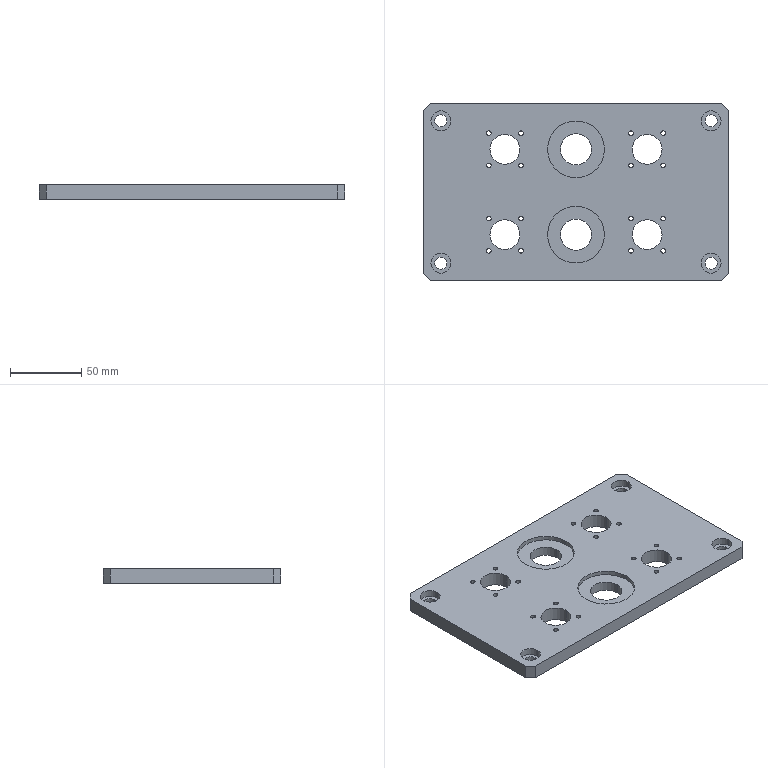CAM job | NX | 3-axis milling, drilling | part box 215 x 125 x 10 mm | stock box 215 x 125 x 10 mm
Tools:
number,name,description,diameter,corner_radius,flute_length,length,flutes
20,ZXZ,Milling Tool-5 Parameters,6.0,0.0,50.0,75.0,2
18,8.5ZT,Drilling Tool,8.5,0.0,35.0,50.0,2
13,3.3ZT,Drilling Tool,3.3,0.0,35.0,50.0,2
17,D17R0.8,Milling Tool-5 Parameters,17.0,0.8,50.0,75.0,2
3,D10,Milling Tool-5 Parameters,10.0,0.0,50.0,75.0,2
4,D10JING,Milling Tool-5 Parameters,10.0,0.0,50.0,75.0,2
2,D6A45,Milling Tool-5 Parameters,6.0,0.0,3.0,3.0,2
Operations:
program,operation,operation_type,tool,method,geometry_group,spindle_rpm,surface_speed,feed_per_tooth,feed_cut,feed_plunge,cut_length_mm,path_length_mm,cut_time_min,machine_time_min
1-215-125-10毛胚,DRILLING_COPY_1,Operation,ZXZ,METHOD,A,3000.0,56.0,0.0333,200.0,0.0,104.0,1041.198,0.52,0.6137
1-215-125-10毛胚,DRILLING_COPY_1_COPY_COPY_COPY_COPY,Operation,8.5ZT,METHOD,A,1200.0,33.0,0.0625,150.0,0.0,160.537,905.82,1.07,1.145
1-215-125-10毛胚,DRILLING_COPY_1_COPY_COPY_COPY_COPY_COPY_1,Operation,3.3ZT,METHOD,A,2000.0,20.0,0.025,100.0,0.0,247.863,1027.047,2.479,2.557
1-215-125-10毛胚,HOLE_MILLING,CylinderMilling,D17R0.8,METHOD,A,2000.0,106.0,0.5,2000.0,100.0,3788.934,4570.656,1.895,1.973
1-215-125-10毛胚,HOLE_MILLING_COPY,CylinderMilling,D17R0.8,METHOD,A,2000.0,106.0,0.5,2000.0,100.0,899.921,1106.921,0.45,0.4707
1-215-125-10毛胚,ZLEVEL_PROFILE_1_COPY_COPY_COPY_COPY,ZLevelMilling,D17R0.8,METHOD,A,2000.0,106.0,0.5,2000.0,2000.0,2329.486,3146.966,1.165,1.246
1-215-125-10毛胚,HOLE_MILLING_COPY_1,CylinderMilling,D10,METHOD,A,3000.0,94.0,0.3333,2000.0,100.0,1384.998,2032.998,0.6925,0.7573
1-215-125-10毛胚,ZLEVEL_PROFILE_COPY_COPY_1_COPY_COPY_COPY_1_COPY,ZLevelMilling,D10JING,METHOD,A,5000.0,157.0,0.1,1000.0,100.0,126.755,1326.76,0.1268,0.2468
1-215-125-10毛胚,FLOOR_WALL_1_COPY_1,VolumeBased25DMillingOperation,D10JING,METHOD,A,5000.0,157.0,0.1,1000.0,100.0,484.905,690.251,0.4849,0.5054
1-215-125-10毛胚,ZLEVEL_PROFILE_COPY_1_COPY_COPY_COPY_COPY_2_COPY,ZLevelMilling,D6A45,METHOD,A,4000.0,75.0,0.125,1000.0,1000.0,1437.348,5667.025,1.437,1.86
1-215-125-10毛胚,ZLEVEL_PROFILE_COPY_1_COPY_COPY_COPY_COPY_2_COPY_COPY,ZLevelMilling,D6A45,METHOD,A,4000.0,75.0,0.125,1000.0,1000.0,133.159,346.71,0.1332,0.1545
1-215-125-10毛胚,ZLEVEL_PROFILE_COPY_1_COPY_COPY_COPY_COPY_2_COPY_COPY_COPY,ZLevelMilling,D6A45,METHOD,A,4000.0,75.0,0.125,1000.0,1000.0,100.26,787.182,0.1003,0.169
1-215-125-10毛胚,刀补4,ZLevelMilling,D10JING,METHOD,A,5000.0,157.0,0.08,800.0,100.0,160.452,706.559,0.2006,0.2552
1-215-125-10毛胚,刀补4_COPY,ZLevelMilling,D10JING,METHOD,A,5000.0,157.0,0.08,800.0,100.0,71.298,737.211,0.0891,0.1557